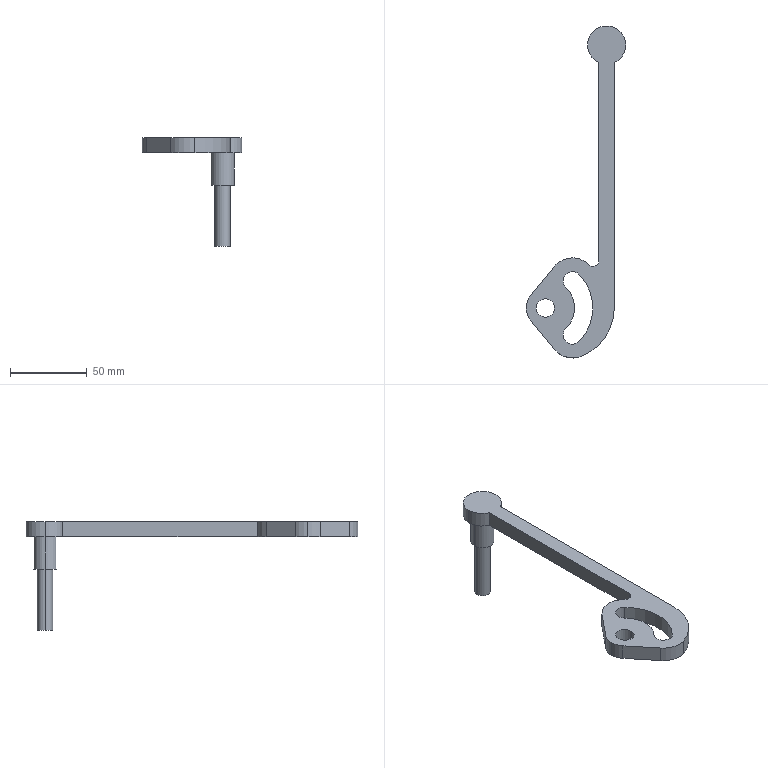Part | SolidWorks | features ICE 2, Extrusion 1 | 1 solid | 29 faces | box 65 x 216.634 x 71 mm | volume 45722 mm3 | cylinder 21 | plane 8 | commonest cylinder face diameters 12 x6 25 x5 10 x2 15 x2 30 x2 7.868 x1
STEP:
#1=CARTESIAN_POINT('',(35.,171.456,-61.));
#2=VERTEX_POINT('',#1);
#3=CARTESIAN_POINT('',(45.,171.456,-61.));
#4=VERTEX_POINT('',#3);
#5=CARTESIAN_POINT('',(40.,171.456,-61.));
#6=DIRECTION('',(0.,0.,-1.));
#7=DIRECTION('',(-1.,0.,0.));
#8=AXIS2_PLACEMENT_3D('',#5,#6,#7);
#9=CIRCLE('',#8,5.);
#10=EDGE_CURVE('',#2,#4,#9,.T.);
#11=ORIENTED_EDGE('',*,*,#10,.F.);
#12=CARTESIAN_POINT('',(35.,171.456,-21.));
#13=VERTEX_POINT('',#12);
#14=CARTESIAN_POINT('',(35.,171.456,-61.));
#15=DIRECTION('',(0.,0.,1.));
#16=VECTOR('',#15,1000.);
#17=LINE('',#14,#16);
#18=EDGE_CURVE('',#2,#13,#17,.T.);
#19=ORIENTED_EDGE('',*,*,#18,.T.);
#20=CARTESIAN_POINT('',(45.,171.456,-21.));
#21=VERTEX_POINT('',#20);
#22=CARTESIAN_POINT('',(40.,171.456,-21.));
#23=DIRECTION('',(0.,0.,-1.));
#24=DIRECTION('',(-1.,0.,0.));
#25=AXIS2_PLACEMENT_3D('',#22,#23,#24);
#26=CIRCLE('',#25,5.);
#27=EDGE_CURVE('',#13,#21,#26,.T.);
#28=ORIENTED_EDGE('',*,*,#27,.T.);
#29=CARTESIAN_POINT('',(45.,171.456,-61.));
#30=DIRECTION('',(0.,0.,1.));
#31=VECTOR('',#30,1000.);
#32=LINE('',#29,#31);
#33=EDGE_CURVE('',#4,#21,#32,.T.);
#34=ORIENTED_EDGE('',*,*,#33,.F.);
#35=EDGE_LOOP('',(#11,#19,#28,#34));
#36=FACE_OUTER_BOUND('',#35,.T.);
#37=CARTESIAN_POINT('',(40.,171.456,-61.));
#38=DIRECTION('',(0.,0.,1.));
#39=DIRECTION('',(1.,0.,0.));
#40=AXIS2_PLACEMENT_3D('',#37,#38,#39);
#41=CYLINDRICAL_SURFACE('',#40,5.);
#42=ADVANCED_FACE('',(#36),#41,.T.);
#43=CARTESIAN_POINT('',(32.5,171.456,-21.));
#44=VERTEX_POINT('',#43);
#45=CARTESIAN_POINT('',(47.5,171.456,-21.));
#46=VERTEX_POINT('',#45);
#47=CARTESIAN_POINT('',(40.,171.456,-21.));
#48=DIRECTION('',(0.,0.,-1.));
#49=DIRECTION('',(-1.,0.,0.));
#50=AXIS2_PLACEMENT_3D('',#47,#48,#49);
#51=CIRCLE('',#50,7.5);
#52=EDGE_CURVE('',#44,#46,#51,.T.);
#53=ORIENTED_EDGE('',*,*,#52,.F.);
#54=CARTESIAN_POINT('',(32.5,171.456,0.));
#55=VERTEX_POINT('',#54);
#56=CARTESIAN_POINT('',(32.5,171.456,-21.));
#57=DIRECTION('',(0.,0.,1.));
#58=VECTOR('',#57,1000.);
#59=LINE('',#56,#58);
#60=EDGE_CURVE('',#44,#55,#59,.T.);
#61=ORIENTED_EDGE('',*,*,#60,.T.);
#62=CARTESIAN_POINT('',(47.5,171.456,0.));
#63=VERTEX_POINT('',#62);
#64=CARTESIAN_POINT('',(40.,171.456,0.));
#65=DIRECTION('',(0.,0.,-1.));
#66=DIRECTION('',(1.,0.,0.));
#67=AXIS2_PLACEMENT_3D('',#64,#65,#66);
#68=CIRCLE('',#67,7.5);
#69=EDGE_CURVE('',#55,#63,#68,.T.);
#70=ORIENTED_EDGE('',*,*,#69,.T.);
#71=CARTESIAN_POINT('',(47.5,171.456,-21.));
#72=DIRECTION('',(0.,0.,1.));
#73=VECTOR('',#72,1000.);
#74=LINE('',#71,#73);
#75=EDGE_CURVE('',#46,#63,#74,.T.);
#76=ORIENTED_EDGE('',*,*,#75,.F.);
#77=EDGE_LOOP('',(#53,#61,#70,#76));
#78=FACE_OUTER_BOUND('',#77,.T.);
#79=CARTESIAN_POINT('',(40.,171.456,-21.));
#80=DIRECTION('',(0.,0.,1.));
#81=DIRECTION('',(1.,0.,0.));
#82=AXIS2_PLACEMENT_3D('',#79,#80,#81);
#83=CYLINDRICAL_SURFACE('',#82,7.5);
#84=ADVANCED_FACE('',(#78),#83,.T.);
#85=CARTESIAN_POINT('',(21.92,21.92,10.));
#86=VERTEX_POINT('',#85);
#87=CARTESIAN_POINT('',(11.678,17.678,10.));
#88=VERTEX_POINT('',#87);
#89=CARTESIAN_POINT('',(17.678,17.678,10.));
#90=DIRECTION('',(0.,0.,1.));
#91=DIRECTION('',(1.,0.,0.));
#92=AXIS2_PLACEMENT_3D('',#89,#90,#91);
#93=CIRCLE('',#92,6.);
#94=EDGE_CURVE('',#86,#88,#93,.T.);
#95=ORIENTED_EDGE('',*,*,#94,.T.);
#96=CARTESIAN_POINT('',(11.678,17.678,0.));
#97=VERTEX_POINT('',#96);
#98=CARTESIAN_POINT('',(11.678,17.678,10.));
#99=DIRECTION('',(0.,0.,-1.));
#100=VECTOR('',#99,1000.);
#101=LINE('',#98,#100);
#102=EDGE_CURVE('',#88,#97,#101,.T.);
#103=ORIENTED_EDGE('',*,*,#102,.T.);
#104=CARTESIAN_POINT('',(21.92,21.92,0.));
#105=VERTEX_POINT('',#104);
#106=CARTESIAN_POINT('',(17.678,17.678,0.));
#107=DIRECTION('',(0.,0.,1.));
#108=DIRECTION('',(1.,0.,0.));
#109=AXIS2_PLACEMENT_3D('',#106,#107,#108);
#110=CIRCLE('',#109,6.);
#111=EDGE_CURVE('',#105,#97,#110,.T.);
#112=ORIENTED_EDGE('',*,*,#111,.F.);
#113=CARTESIAN_POINT('',(21.92,21.92,10.));
#114=DIRECTION('',(0.,0.,-1.));
#115=VECTOR('',#114,1000.);
#116=LINE('',#113,#115);
#117=EDGE_CURVE('',#86,#105,#116,.T.);
#118=ORIENTED_EDGE('',*,*,#117,.F.);
#119=EDGE_LOOP('',(#95,#103,#112,#118));
#120=FACE_OUTER_BOUND('',#119,.T.);
#121=CARTESIAN_POINT('',(17.678,17.678,10.));
#122=DIRECTION('',(0.,0.,-1.));
#123=DIRECTION('',(-1.,0.,0.));
#124=AXIS2_PLACEMENT_3D('',#121,#122,#123);
#125=CYLINDRICAL_SURFACE('',#124,6.);
#126=ADVANCED_FACE('',(#120),#125,.F.);
#127=CARTESIAN_POINT('',(13.435,-13.435,10.));
#128=VERTEX_POINT('',#127);
#129=CARTESIAN_POINT('',(11.678,-17.678,10.));
#130=VERTEX_POINT('',#129);
#131=CARTESIAN_POINT('',(17.678,-17.678,10.));
#132=DIRECTION('',(0.,0.,1.));
#133=DIRECTION('',(1.,0.,0.));
#134=AXIS2_PLACEMENT_3D('',#131,#132,#133);
#135=CIRCLE('',#134,6.);
#136=EDGE_CURVE('',#128,#130,#135,.T.);
#137=ORIENTED_EDGE('',*,*,#136,.T.);
#138=CARTESIAN_POINT('',(11.678,-17.678,0.));
#139=VERTEX_POINT('',#138);
#140=CARTESIAN_POINT('',(11.678,-17.678,10.));
#141=DIRECTION('',(0.,0.,-1.));
#142=VECTOR('',#141,1000.);
#143=LINE('',#140,#142);
#144=EDGE_CURVE('',#130,#139,#143,.T.);
#145=ORIENTED_EDGE('',*,*,#144,.T.);
#146=CARTESIAN_POINT('',(13.435,-13.435,0.));
#147=VERTEX_POINT('',#146);
#148=CARTESIAN_POINT('',(17.678,-17.678,0.));
#149=DIRECTION('',(0.,0.,1.));
#150=DIRECTION('',(1.,0.,0.));
#151=AXIS2_PLACEMENT_3D('',#148,#149,#150);
#152=CIRCLE('',#151,6.);
#153=EDGE_CURVE('',#147,#139,#152,.T.);
#154=ORIENTED_EDGE('',*,*,#153,.F.);
#155=CARTESIAN_POINT('',(13.435,-13.435,10.));
#156=DIRECTION('',(0.,0.,-1.));
#157=VECTOR('',#156,1000.);
#158=LINE('',#155,#157);
#159=EDGE_CURVE('',#128,#147,#158,.T.);
#160=ORIENTED_EDGE('',*,*,#159,.F.);
#161=EDGE_LOOP('',(#137,#145,#154,#160));
#162=FACE_OUTER_BOUND('',#161,.T.);
#163=CARTESIAN_POINT('',(17.678,-17.678,10.));
#164=DIRECTION('',(0.,0.,-1.));
#165=DIRECTION('',(-1.,0.,0.));
#166=AXIS2_PLACEMENT_3D('',#163,#164,#165);
#167=CYLINDRICAL_SURFACE('',#166,6.);
#168=ADVANCED_FACE('',(#162),#167,.F.);
#169=CARTESIAN_POINT('',(-6.,0.,10.));
#170=VERTEX_POINT('',#169);
#171=CARTESIAN_POINT('',(6.,0.,10.));
#172=VERTEX_POINT('',#171);
#173=CARTESIAN_POINT('',(0.,0.,10.));
#174=DIRECTION('',(0.,0.,1.));
#175=DIRECTION('',(1.,0.,0.));
#176=AXIS2_PLACEMENT_3D('',#173,#174,#175);
#177=CIRCLE('',#176,6.);
#178=EDGE_CURVE('',#170,#172,#177,.T.);
#179=ORIENTED_EDGE('',*,*,#178,.T.);
#180=CARTESIAN_POINT('',(6.,0.,0.));
#181=VERTEX_POINT('',#180);
#182=CARTESIAN_POINT('',(6.,0.,10.));
#183=DIRECTION('',(0.,0.,-1.));
#184=VECTOR('',#183,1000.);
#185=LINE('',#182,#184);
#186=EDGE_CURVE('',#172,#181,#185,.T.);
#187=ORIENTED_EDGE('',*,*,#186,.T.);
#188=CARTESIAN_POINT('',(-6.,0.,0.));
#189=VERTEX_POINT('',#188);
#190=CARTESIAN_POINT('',(0.,0.,0.));
#191=DIRECTION('',(0.,0.,1.));
#192=DIRECTION('',(1.,0.,0.));
#193=AXIS2_PLACEMENT_3D('',#190,#191,#192);
#194=CIRCLE('',#193,6.);
#195=EDGE_CURVE('',#189,#181,#194,.T.);
#196=ORIENTED_EDGE('',*,*,#195,.F.);
#197=CARTESIAN_POINT('',(-6.,0.,10.));
#198=DIRECTION('',(0.,0.,-1.));
#199=VECTOR('',#198,1000.);
#200=LINE('',#197,#199);
#201=EDGE_CURVE('',#170,#189,#200,.T.);
#202=ORIENTED_EDGE('',*,*,#201,.F.);
#203=EDGE_LOOP('',(#179,#187,#196,#202));
#204=FACE_OUTER_BOUND('',#203,.T.);
#205=CARTESIAN_POINT('',(0.,0.,10.));
#206=DIRECTION('',(0.,0.,-1.));
#207=DIRECTION('',(-1.,0.,0.));
#208=AXIS2_PLACEMENT_3D('',#205,#206,#207);
#209=CYLINDRICAL_SURFACE('',#208,6.);
#210=ADVANCED_FACE('',(#204),#209,.F.);
#211=CARTESIAN_POINT('',(52.5,171.456,10.));
#212=VERTEX_POINT('',#211);
#213=CARTESIAN_POINT('',(27.5,171.456,10.));
#214=VERTEX_POINT('',#213);
#215=CARTESIAN_POINT('',(40.,171.456,10.));
#216=DIRECTION('',(0.,0.,1.));
#217=DIRECTION('',(1.,0.,0.));
#218=AXIS2_PLACEMENT_3D('',#215,#216,#217);
#219=CIRCLE('',#218,12.5);
#220=EDGE_CURVE('',#212,#214,#219,.T.);
#221=ORIENTED_EDGE('',*,*,#220,.F.);
#222=CARTESIAN_POINT('',(52.5,171.456,0.));
#223=VERTEX_POINT('',#222);
#224=CARTESIAN_POINT('',(52.5,171.456,10.));
#225=DIRECTION('',(0.,0.,-1.));
#226=VECTOR('',#225,1000.);
#227=LINE('',#224,#226);
#228=EDGE_CURVE('',#212,#223,#227,.T.);
#229=ORIENTED_EDGE('',*,*,#228,.T.);
#230=CARTESIAN_POINT('',(27.5,171.456,0.));
#231=VERTEX_POINT('',#230);
#232=CARTESIAN_POINT('',(40.,171.456,0.));
#233=DIRECTION('',(0.,0.,1.));
#234=DIRECTION('',(1.,0.,0.));
#235=AXIS2_PLACEMENT_3D('',#232,#233,#234);
#236=CIRCLE('',#235,12.5);
#237=EDGE_CURVE('',#223,#231,#236,.T.);
#238=ORIENTED_EDGE('',*,*,#237,.T.);
#239=CARTESIAN_POINT('',(27.5,171.456,10.));
#240=DIRECTION('',(0.,0.,-1.));
#241=VECTOR('',#240,1000.);
#242=LINE('',#239,#241);
#243=EDGE_CURVE('',#214,#231,#242,.T.);
#244=ORIENTED_EDGE('',*,*,#243,.F.);
#245=EDGE_LOOP('',(#221,#229,#238,#244));
#246=FACE_OUTER_BOUND('',#245,.T.);
#247=CARTESIAN_POINT('',(40.,171.456,10.));
#248=DIRECTION('',(0.,0.,-1.));
#249=DIRECTION('',(-1.,0.,0.));
#250=AXIS2_PLACEMENT_3D('',#247,#248,#249);
#251=CYLINDRICAL_SURFACE('',#250,12.5);
#252=ADVANCED_FACE('',(#246),#251,.T.);
#253=CARTESIAN_POINT('',(35.,160.,10.));
#254=VERTEX_POINT('',#253);
#255=CARTESIAN_POINT('',(40.,171.456,10.));
#256=DIRECTION('',(0.,0.,1.));
#257=DIRECTION('',(1.,0.,0.));
#258=AXIS2_PLACEMENT_3D('',#255,#256,#257);
#259=CIRCLE('',#258,12.5);
#260=EDGE_CURVE('',#214,#254,#259,.T.);
#261=ORIENTED_EDGE('',*,*,#260,.F.);
#262=ORIENTED_EDGE('',*,*,#243,.T.);
#263=CARTESIAN_POINT('',(35.,160.,0.));
#264=VERTEX_POINT('',#263);
#265=CARTESIAN_POINT('',(40.,171.456,0.));
#266=DIRECTION('',(0.,0.,1.));
#267=DIRECTION('',(1.,0.,0.));
#268=AXIS2_PLACEMENT_3D('',#265,#266,#267);
#269=CIRCLE('',#268,12.5);
#270=EDGE_CURVE('',#231,#264,#269,.T.);
#271=ORIENTED_EDGE('',*,*,#270,.T.);
#272=CARTESIAN_POINT('',(35.,160.,10.));
#273=DIRECTION('',(0.,0.,-1.));
#274=VECTOR('',#273,1000.);
#275=LINE('',#272,#274);
#276=EDGE_CURVE('',#254,#264,#275,.T.);
#277=ORIENTED_EDGE('',*,*,#276,.F.);
#278=EDGE_LOOP('',(#261,#262,#271,#277));
#279=FACE_OUTER_BOUND('',#278,.T.);
#280=CARTESIAN_POINT('',(40.,171.456,10.));
#281=DIRECTION('',(0.,0.,-1.));
#282=DIRECTION('',(-1.,0.,0.));
#283=AXIS2_PLACEMENT_3D('',#280,#281,#282);
#284=CYLINDRICAL_SURFACE('',#283,12.5);
#285=ADVANCED_FACE('',(#279),#284,.T.);
#286=CARTESIAN_POINT('',(-12.5,0.,10.));
#287=VERTEX_POINT('',#286);
#288=CARTESIAN_POINT('',(-9.678,-7.911,10.));
#289=VERTEX_POINT('',#288);
#290=CARTESIAN_POINT('',(0.,0.,10.));
#291=DIRECTION('',(0.,0.,1.));
#292=DIRECTION('',(1.,0.,0.));
#293=AXIS2_PLACEMENT_3D('',#290,#291,#292);
#294=CIRCLE('',#293,12.5);
#295=EDGE_CURVE('',#287,#289,#294,.T.);
#296=ORIENTED_EDGE('',*,*,#295,.F.);
#297=CARTESIAN_POINT('',(-12.5,0.,0.));
#298=VERTEX_POINT('',#297);
#299=CARTESIAN_POINT('',(-12.5,0.,10.));
#300=DIRECTION('',(0.,0.,-1.));
#301=VECTOR('',#300,1000.);
#302=LINE('',#299,#301);
#303=EDGE_CURVE('',#287,#298,#302,.T.);
#304=ORIENTED_EDGE('',*,*,#303,.T.);
#305=CARTESIAN_POINT('',(-9.678,-7.911,0.));
#306=VERTEX_POINT('',#305);
#307=CARTESIAN_POINT('',(0.,0.,0.));
#308=DIRECTION('',(0.,0.,1.));
#309=DIRECTION('',(1.,0.,0.));
#310=AXIS2_PLACEMENT_3D('',#307,#308,#309);
#311=CIRCLE('',#310,12.5);
#312=EDGE_CURVE('',#298,#306,#311,.T.);
#313=ORIENTED_EDGE('',*,*,#312,.T.);
#314=CARTESIAN_POINT('',(-9.678,-7.911,10.));
#315=DIRECTION('',(0.,0.,-1.));
#316=VECTOR('',#315,1000.);
#317=LINE('',#314,#316);
#318=EDGE_CURVE('',#289,#306,#317,.T.);
#319=ORIENTED_EDGE('',*,*,#318,.F.);
#320=EDGE_LOOP('',(#296,#304,#313,#319));
#321=FACE_OUTER_BOUND('',#320,.T.);
#322=CARTESIAN_POINT('',(0.,0.,10.));
#323=DIRECTION('',(0.,0.,-1.));
#324=DIRECTION('',(-1.,0.,0.));
#325=AXIS2_PLACEMENT_3D('',#322,#323,#324);
#326=CYLINDRICAL_SURFACE('',#325,12.5);
#327=ADVANCED_FACE('',(#321),#326,.T.);
#328=CARTESIAN_POINT('',(40.,171.456,-21.));
#329=DIRECTION('',(0.,0.,-1.));
#330=DIRECTION('',(-1.,0.,0.));
#331=AXIS2_PLACEMENT_3D('',#328,#329,#330);
#332=CIRCLE('',#331,7.5);
#333=EDGE_CURVE('',#46,#44,#332,.T.);
#334=ORIENTED_EDGE('',*,*,#333,.T.);
#335=ORIENTED_EDGE('',*,*,#52,.T.);
#336=EDGE_LOOP('',(#334,#335));
#337=FACE_OUTER_BOUND('',#336,.T.);
#338=CARTESIAN_POINT('',(40.,171.456,-21.));
#339=DIRECTION('',(0.,0.,-1.));
#340=DIRECTION('',(-1.,0.,0.));
#341=AXIS2_PLACEMENT_3D('',#338,#339,#340);
#342=CIRCLE('',#341,5.);
#343=EDGE_CURVE('',#21,#13,#342,.T.);
#344=ORIENTED_EDGE('',*,*,#343,.F.);
#345=ORIENTED_EDGE('',*,*,#27,.F.);
#346=EDGE_LOOP('',(#344,#345));
#347=FACE_BOUND('',#346,.T.);
#348=CARTESIAN_POINT('',(40.,171.456,-21.));
#349=DIRECTION('',(0.,0.,-1.));
#350=DIRECTION('',(-1.,0.,0.));
#351=AXIS2_PLACEMENT_3D('',#348,#349,#350);
#352=PLANE('',#351);
#353=ADVANCED_FACE('',(#337,#347),#352,.T.);
#354=ORIENTED_EDGE('',*,*,#153,.T.);
#355=CARTESIAN_POINT('',(21.92,-21.92,0.));
#356=VERTEX_POINT('',#355);
#357=CARTESIAN_POINT('',(17.678,-17.678,0.));
#358=DIRECTION('',(0.,0.,1.));
#359=DIRECTION('',(1.,0.,0.));
#360=AXIS2_PLACEMENT_3D('',#357,#358,#359);
#361=CIRCLE('',#360,6.);
#362=EDGE_CURVE('',#139,#356,#361,.T.);
#363=ORIENTED_EDGE('',*,*,#362,.T.);
#364=CARTESIAN_POINT('',(0.,0.,0.));
#365=DIRECTION('',(0.,0.,1.));
#366=DIRECTION('',(1.,0.,0.));
#367=AXIS2_PLACEMENT_3D('',#364,#365,#366);
#368=CIRCLE('',#367,31.);
#369=EDGE_CURVE('',#356,#105,#368,.T.);
#370=ORIENTED_EDGE('',*,*,#369,.T.);
#371=ORIENTED_EDGE('',*,*,#111,.T.);
#372=CARTESIAN_POINT('',(13.435,13.435,0.));
#373=VERTEX_POINT('',#372);
#374=CARTESIAN_POINT('',(17.678,17.678,0.));
#375=DIRECTION('',(0.,0.,1.));
#376=DIRECTION('',(1.,0.,0.));
#377=AXIS2_PLACEMENT_3D('',#374,#375,#376);
#378=CIRCLE('',#377,6.);
#379=EDGE_CURVE('',#97,#373,#378,.T.);
#380=ORIENTED_EDGE('',*,*,#379,.T.);
#381=CARTESIAN_POINT('',(0.,0.,0.));
#382=DIRECTION('',(0.,0.,-1.));
#383=DIRECTION('',(1.,0.,0.));
#384=AXIS2_PLACEMENT_3D('',#381,#382,#383);
#385=CIRCLE('',#384,19.);
#386=EDGE_CURVE('',#373,#147,#385,.T.);
#387=ORIENTED_EDGE('',*,*,#386,.T.);
#388=EDGE_LOOP('',(#354,#363,#370,#371,#380,#387));
#389=FACE_BOUND('',#388,.T.);
#390=CARTESIAN_POINT('',(35.,31.066,0.));
#391=VERTEX_POINT('',#390);
#392=CARTESIAN_POINT('',(28.284,28.284,0.));
#393=VERTEX_POINT('',#392);
#394=CARTESIAN_POINT('',(31.066,31.066,0.));
#395=DIRECTION('',(0.,0.,-1.));
#396=DIRECTION('',(1.,0.,0.));
#397=AXIS2_PLACEMENT_3D('',#394,#395,#396);
#398=CIRCLE('',#397,3.934);
#399=EDGE_CURVE('',#391,#393,#398,.T.);
#400=ORIENTED_EDGE('',*,*,#399,.F.);
#401=CARTESIAN_POINT('',(35.,160.,0.));
#402=DIRECTION('',(0.,-1.,0.));
#403=VECTOR('',#402,1000.);
#404=LINE('',#401,#403);
#405=EDGE_CURVE('',#264,#391,#404,.T.);
#406=ORIENTED_EDGE('',*,*,#405,.F.);
#407=ORIENTED_EDGE('',*,*,#270,.F.);
#408=ORIENTED_EDGE('',*,*,#237,.F.);
#409=CARTESIAN_POINT('',(45.,160.,0.));
#410=VERTEX_POINT('',#409);
#411=CARTESIAN_POINT('',(40.,171.456,0.));
#412=DIRECTION('',(0.,0.,1.));
#413=DIRECTION('',(1.,0.,0.));
#414=AXIS2_PLACEMENT_3D('',#411,#412,#413);
#415=CIRCLE('',#414,12.5);
#416=EDGE_CURVE('',#410,#223,#415,.T.);
#417=ORIENTED_EDGE('',*,*,#416,.F.);
#418=CARTESIAN_POINT('',(45.,0.,0.));
#419=VERTEX_POINT('',#418);
#420=CARTESIAN_POINT('',(45.,0.,0.));
#421=DIRECTION('',(0.,1.,0.));
#422=VECTOR('',#421,1000.);
#423=LINE('',#420,#422);
#424=EDGE_CURVE('',#419,#410,#423,.T.);
#425=ORIENTED_EDGE('',*,*,#424,.F.);
#426=CARTESIAN_POINT('',(21.92,-32.065,0.));
#427=VERTEX_POINT('',#426);
#428=CARTESIAN_POINT('',(11.186,0.,0.));
#429=DIRECTION('',(0.,0.,1.));
#430=DIRECTION('',(-1.,0.,0.));
#431=AXIS2_PLACEMENT_3D('',#428,#429,#430);
#432=CIRCLE('',#431,33.814);
#433=EDGE_CURVE('',#427,#419,#432,.T.);
#434=ORIENTED_EDGE('',*,*,#433,.F.);
#435=CARTESIAN_POINT('',(6.064,-27.17,0.));
#436=VERTEX_POINT('',#435);
#437=CARTESIAN_POINT('',(17.678,-17.678,0.));
#438=DIRECTION('',(0.,0.,1.));
#439=DIRECTION('',(1.,0.,0.));
#440=AXIS2_PLACEMENT_3D('',#437,#438,#439);
#441=CIRCLE('',#440,15.);
#442=EDGE_CURVE('',#436,#427,#441,.T.);
#443=ORIENTED_EDGE('',*,*,#442,.F.);
#444=CARTESIAN_POINT('',(-9.678,-7.911,0.));
#445=DIRECTION('',(0.6329,-0.7743,0.));
#446=VECTOR('',#445,1000.);
#447=LINE('',#444,#446);
#448=EDGE_CURVE('',#306,#436,#447,.T.);
#449=ORIENTED_EDGE('',*,*,#448,.F.);
#450=ORIENTED_EDGE('',*,*,#312,.F.);
#451=CARTESIAN_POINT('',(-9.678,7.911,0.));
#452=VERTEX_POINT('',#451);
#453=CARTESIAN_POINT('',(0.,0.,0.));
#454=DIRECTION('',(0.,0.,1.));
#455=DIRECTION('',(1.,0.,0.));
#456=AXIS2_PLACEMENT_3D('',#453,#454,#455);
#457=CIRCLE('',#456,12.5);
#458=EDGE_CURVE('',#452,#298,#457,.T.);
#459=ORIENTED_EDGE('',*,*,#458,.F.);
#460=CARTESIAN_POINT('',(6.064,27.17,0.));
#461=VERTEX_POINT('',#460);
#462=CARTESIAN_POINT('',(-9.678,7.911,0.));
#463=DIRECTION('',(-0.6329,-0.7743,0.));
#464=VECTOR('',#463,1000.);
#465=LINE('',#462,#464);
#466=EDGE_CURVE('',#461,#452,#465,.T.);
#467=ORIENTED_EDGE('',*,*,#466,.F.);
#468=CARTESIAN_POINT('',(17.678,17.678,0.));
#469=DIRECTION('',(0.,0.,1.));
#470=DIRECTION('',(1.,0.,0.));
#471=AXIS2_PLACEMENT_3D('',#468,#469,#470);
#472=CIRCLE('',#471,15.);
#473=EDGE_CURVE('',#393,#461,#472,.T.);
#474=ORIENTED_EDGE('',*,*,#473,.F.);
#475=EDGE_LOOP('',(#400,#406,#407,#408,#417,#425,#434,#443,#449,#450,#459,#467,#474));
#476=FACE_OUTER_BOUND('',#475,.T.);
#477=ORIENTED_EDGE('',*,*,#195,.T.);
#478=CARTESIAN_POINT('',(0.,0.,0.));
#479=DIRECTION('',(0.,0.,1.));
#480=DIRECTION('',(1.,0.,0.));
#481=AXIS2_PLACEMENT_3D('',#478,#479,#480);
#482=CIRCLE('',#481,6.);
#483=EDGE_CURVE('',#181,#189,#482,.T.);
#484=ORIENTED_EDGE('',*,*,#483,.T.);
#485=EDGE_LOOP('',(#477,#484));
#486=FACE_BOUND('',#485,.T.);
#487=CARTESIAN_POINT('',(40.,171.456,0.));
#488=DIRECTION('',(0.,0.,-1.));
#489=DIRECTION('',(1.,0.,0.));
#490=AXIS2_PLACEMENT_3D('',#487,#488,#489);
#491=CIRCLE('',#490,7.5);
#492=EDGE_CURVE('',#63,#55,#491,.T.);
#493=ORIENTED_EDGE('',*,*,#492,.F.);
#494=ORIENTED_EDGE('',*,*,#69,.F.);
#495=EDGE_LOOP('',(#493,#494));
#496=FACE_BOUND('',#495,.T.);
#497=CARTESIAN_POINT('',(31.066,31.066,0.));
#498=DIRECTION('',(0.,0.,1.));
#499=DIRECTION('',(1.,0.,0.));
#500=AXIS2_PLACEMENT_3D('',#497,#498,#499);
#501=PLANE('',#500);
#502=ADVANCED_FACE('',(#389,#476,#486,#496),#501,.F.);
#503=ORIENTED_EDGE('',*,*,#178,.F.);
#504=CARTESIAN_POINT('',(0.,0.,10.));
#505=DIRECTION('',(0.,0.,1.));
#506=DIRECTION('',(1.,0.,0.));
#507=AXIS2_PLACEMENT_3D('',#504,#505,#506);
#508=CIRCLE('',#507,6.);
#509=EDGE_CURVE('',#172,#170,#508,.T.);
#510=ORIENTED_EDGE('',*,*,#509,.F.);
#511=EDGE_LOOP('',(#503,#510));
#512=FACE_BOUND('',#511,.T.);
#513=CARTESIAN_POINT('',(35.,31.066,10.));
#514=VERTEX_POINT('',#513);
#515=CARTESIAN_POINT('',(28.284,28.284,10.));
#516=VERTEX_POINT('',#515);
#517=CARTESIAN_POINT('',(31.066,31.066,10.));
#518=DIRECTION('',(0.,0.,-1.));
#519=DIRECTION('',(1.,0.,0.));
#520=AXIS2_PLACEMENT_3D('',#517,#518,#519);
#521=CIRCLE('',#520,3.934);
#522=EDGE_CURVE('',#514,#516,#521,.T.);
#523=ORIENTED_EDGE('',*,*,#522,.T.);
#524=CARTESIAN_POINT('',(6.064,27.17,10.));
#525=VERTEX_POINT('',#524);
#526=CARTESIAN_POINT('',(17.678,17.678,10.));
#527=DIRECTION('',(0.,0.,1.));
#528=DIRECTION('',(1.,0.,0.));
#529=AXIS2_PLACEMENT_3D('',#526,#527,#528);
#530=CIRCLE('',#529,15.);
#531=EDGE_CURVE('',#516,#525,#530,.T.);
#532=ORIENTED_EDGE('',*,*,#531,.T.);
#533=CARTESIAN_POINT('',(-9.678,7.911,10.));
#534=VERTEX_POINT('',#533);
#535=CARTESIAN_POINT('',(-9.678,7.911,10.));
#536=DIRECTION('',(-0.6329,-0.7743,0.));
#537=VECTOR('',#536,1000.);
#538=LINE('',#535,#537);
#539=EDGE_CURVE('',#525,#534,#538,.T.);
#540=ORIENTED_EDGE('',*,*,#539,.T.);
#541=CARTESIAN_POINT('',(0.,0.,10.));
#542=DIRECTION('',(0.,0.,1.));
#543=DIRECTION('',(1.,0.,0.));
#544=AXIS2_PLACEMENT_3D('',#541,#542,#543);
#545=CIRCLE('',#544,12.5);
#546=EDGE_CURVE('',#534,#287,#545,.T.);
#547=ORIENTED_EDGE('',*,*,#546,.T.);
#548=ORIENTED_EDGE('',*,*,#295,.T.);
#549=CARTESIAN_POINT('',(6.064,-27.17,10.));
#550=VERTEX_POINT('',#549);
#551=CARTESIAN_POINT('',(-9.678,-7.911,10.));
#552=DIRECTION('',(0.6329,-0.7743,0.));
#553=VECTOR('',#552,1000.);
#554=LINE('',#551,#553);
#555=EDGE_CURVE('',#289,#550,#554,.T.);
#556=ORIENTED_EDGE('',*,*,#555,.T.);
#557=CARTESIAN_POINT('',(21.92,-32.065,10.));
#558=VERTEX_POINT('',#557);
#559=CARTESIAN_POINT('',(17.678,-17.678,10.));
#560=DIRECTION('',(0.,0.,1.));
#561=DIRECTION('',(1.,0.,0.));
#562=AXIS2_PLACEMENT_3D('',#559,#560,#561);
#563=CIRCLE('',#562,15.);
#564=EDGE_CURVE('',#550,#558,#563,.T.);
#565=ORIENTED_EDGE('',*,*,#564,.T.);
#566=CARTESIAN_POINT('',(45.,0.,10.));
#567=VERTEX_POINT('',#566);
#568=CARTESIAN_POINT('',(11.186,0.,10.));
#569=DIRECTION('',(0.,0.,1.));
#570=DIRECTION('',(-1.,0.,0.));
#571=AXIS2_PLACEMENT_3D('',#568,#569,#570);
#572=CIRCLE('',#571,33.814);
#573=EDGE_CURVE('',#558,#567,#572,.T.);
#574=ORIENTED_EDGE('',*,*,#573,.T.);
#575=CARTESIAN_POINT('',(45.,160.,10.));
#576=VERTEX_POINT('',#575);
#577=CARTESIAN_POINT('',(45.,0.,10.));
#578=DIRECTION('',(0.,1.,0.));
#579=VECTOR('',#578,1000.);
#580=LINE('',#577,#579);
#581=EDGE_CURVE('',#567,#576,#580,.T.);
#582=ORIENTED_EDGE('',*,*,#581,.T.);
#583=CARTESIAN_POINT('',(40.,171.456,10.));
#584=DIRECTION('',(0.,0.,1.));
#585=DIRECTION('',(1.,0.,0.));
#586=AXIS2_PLACEMENT_3D('',#583,#584,#585);
#587=CIRCLE('',#586,12.5);
#588=EDGE_CURVE('',#576,#212,#587,.T.);
#589=ORIENTED_EDGE('',*,*,#588,.T.);
#590=ORIENTED_EDGE('',*,*,#220,.T.);
#591=ORIENTED_EDGE('',*,*,#260,.T.);
#592=CARTESIAN_POINT('',(35.,160.,10.));
#593=DIRECTION('',(0.,-1.,0.));
#594=VECTOR('',#593,1000.);
#595=LINE('',#592,#594);
#596=EDGE_CURVE('',#254,#514,#595,.T.);
#597=ORIENTED_EDGE('',*,*,#596,.T.);
#598=EDGE_LOOP('',(#523,#532,#540,#547,#548,#556,#565,#574,#582,#589,#590,#591,#597));
#599=FACE_OUTER_BOUND('',#598,.T.);
#600=CARTESIAN_POINT('',(21.92,-21.92,10.));
#601=VERTEX_POINT('',#600);
#602=CARTESIAN_POINT('',(0.,0.,10.));
#603=DIRECTION('',(0.,0.,1.));
#604=DIRECTION('',(1.,0.,0.));
#605=AXIS2_PLACEMENT_3D('',#602,#603,#604);
#606=CIRCLE('',#605,31.);
#607=EDGE_CURVE('',#601,#86,#606,.T.);
#608=ORIENTED_EDGE('',*,*,#607,.F.);
#609=CARTESIAN_POINT('',(17.678,-17.678,10.));
#610=DIRECTION('',(0.,0.,1.));
#611=DIRECTION('',(1.,0.,0.));
#612=AXIS2_PLACEMENT_3D('',#609,#610,#611);
#613=CIRCLE('',#612,6.);
#614=EDGE_CURVE('',#130,#601,#613,.T.);
#615=ORIENTED_EDGE('',*,*,#614,.F.);
#616=ORIENTED_EDGE('',*,*,#136,.F.);
#617=CARTESIAN_POINT('',(13.435,13.435,10.));
#618=VERTEX_POINT('',#617);
#619=CARTESIAN_POINT('',(0.,0.,10.));
#620=DIRECTION('',(0.,0.,-1.));
#621=DIRECTION('',(1.,0.,0.));
#622=AXIS2_PLACEMENT_3D('',#619,#620,#621);
#623=CIRCLE('',#622,19.);
#624=EDGE_CURVE('',#618,#128,#623,.T.);
#625=ORIENTED_EDGE('',*,*,#624,.F.);
#626=CARTESIAN_POINT('',(17.678,17.678,10.));
#627=DIRECTION('',(0.,0.,1.));
#628=DIRECTION('',(1.,0.,0.));
#629=AXIS2_PLACEMENT_3D('',#626,#627,#628);
#630=CIRCLE('',#629,6.);
#631=EDGE_CURVE('',#88,#618,#630,.T.);
#632=ORIENTED_EDGE('',*,*,#631,.F.);
#633=ORIENTED_EDGE('',*,*,#94,.F.);
#634=EDGE_LOOP('',(#608,#615,#616,#625,#632,#633));
#635=FACE_BOUND('',#634,.T.);
#636=CARTESIAN_POINT('',(31.066,31.066,10.));
#637=DIRECTION('',(0.,0.,1.));
#638=DIRECTION('',(1.,0.,0.));
#639=AXIS2_PLACEMENT_3D('',#636,#637,#638);
#640=PLANE('',#639);
#641=ADVANCED_FACE('',(#512,#599,#635),#640,.T.);
#642=ORIENTED_EDGE('',*,*,#399,.T.);
#643=CARTESIAN_POINT('',(28.284,28.284,10.));
#644=DIRECTION('',(0.,0.,-1.));
#645=VECTOR('',#644,1000.);
#646=LINE('',#643,#645);
#647=EDGE_CURVE('',#516,#393,#646,.T.);
#648=ORIENTED_EDGE('',*,*,#647,.F.);
#649=ORIENTED_EDGE('',*,*,#522,.F.);
#650=CARTESIAN_POINT('',(35.,31.066,10.));
#651=DIRECTION('',(0.,0.,-1.));
#652=VECTOR('',#651,1000.);
#653=LINE('',#650,#652);
#654=EDGE_CURVE('',#514,#391,#653,.T.);
#655=ORIENTED_EDGE('',*,*,#654,.T.);
#656=EDGE_LOOP('',(#642,#648,#649,#655));
#657=FACE_OUTER_BOUND('',#656,.T.);
#658=CARTESIAN_POINT('',(31.066,31.066,10.));
#659=DIRECTION('',(0.,0.,-1.));
#660=DIRECTION('',(-1.,0.,0.));
#661=AXIS2_PLACEMENT_3D('',#658,#659,#660);
#662=CYLINDRICAL_SURFACE('',#661,3.934);
#663=ADVANCED_FACE('',(#657),#662,.F.);
#664=ORIENTED_EDGE('',*,*,#473,.T.);
#665=CARTESIAN_POINT('',(6.064,27.17,10.));
#666=DIRECTION('',(0.,0.,-1.));
#667=VECTOR('',#666,1000.);
#668=LINE('',#665,#667);
#669=EDGE_CURVE('',#525,#461,#668,.T.);
#670=ORIENTED_EDGE('',*,*,#669,.F.);
#671=ORIENTED_EDGE('',*,*,#531,.F.);
#672=ORIENTED_EDGE('',*,*,#647,.T.);
#673=EDGE_LOOP('',(#664,#670,#671,#672));
#674=FACE_OUTER_BOUND('',#673,.T.);
#675=CARTESIAN_POINT('',(17.678,17.678,10.));
#676=DIRECTION('',(0.,0.,-1.));
#677=DIRECTION('',(-1.,0.,0.));
#678=AXIS2_PLACEMENT_3D('',#675,#676,#677);
#679=CYLINDRICAL_SURFACE('',#678,15.);
#680=ADVANCED_FACE('',(#674),#679,.T.);
#681=ORIENTED_EDGE('',*,*,#466,.T.);
#682=CARTESIAN_POINT('',(-9.678,7.911,10.));
#683=DIRECTION('',(0.,0.,-1.));
#684=VECTOR('',#683,1000.);
#685=LINE('',#682,#684);
#686=EDGE_CURVE('',#534,#452,#685,.T.);
#687=ORIENTED_EDGE('',*,*,#686,.F.);
#688=ORIENTED_EDGE('',*,*,#539,.F.);
#689=ORIENTED_EDGE('',*,*,#669,.T.);
#690=EDGE_LOOP('',(#681,#687,#688,#689));
#691=FACE_OUTER_BOUND('',#690,.T.);
#692=CARTESIAN_POINT('',(-9.678,7.911,10.));
#693=DIRECTION('',(0.7743,-0.6329,0.));
#694=DIRECTION('',(0.6329,0.7743,0.));
#695=AXIS2_PLACEMENT_3D('',#692,#693,#694);
#696=PLANE('',#695);
#697=ADVANCED_FACE('',(#691),#696,.F.);
#698=ORIENTED_EDGE('',*,*,#303,.F.);
#699=ORIENTED_EDGE('',*,*,#546,.F.);
#700=ORIENTED_EDGE('',*,*,#686,.T.);
#701=ORIENTED_EDGE('',*,*,#458,.T.);
#702=EDGE_LOOP('',(#698,#699,#700,#701));
#703=FACE_OUTER_BOUND('',#702,.T.);
#704=CARTESIAN_POINT('',(0.,0.,10.));
#705=DIRECTION('',(0.,0.,-1.));
#706=DIRECTION('',(-1.,0.,0.));
#707=AXIS2_PLACEMENT_3D('',#704,#705,#706);
#708=CYLINDRICAL_SURFACE('',#707,12.5);
#709=ADVANCED_FACE('',(#703),#708,.T.);
#710=ORIENTED_EDGE('',*,*,#448,.T.);
#711=CARTESIAN_POINT('',(6.064,-27.17,10.));
#712=DIRECTION('',(0.,0.,-1.));
#713=VECTOR('',#712,1000.);
#714=LINE('',#711,#713);
#715=EDGE_CURVE('',#550,#436,#714,.T.);
#716=ORIENTED_EDGE('',*,*,#715,.F.);
#717=ORIENTED_EDGE('',*,*,#555,.F.);
#718=ORIENTED_EDGE('',*,*,#318,.T.);
#719=EDGE_LOOP('',(#710,#716,#717,#718));
#720=FACE_OUTER_BOUND('',#719,.T.);
#721=CARTESIAN_POINT('',(-9.678,-7.911,10.));
#722=DIRECTION('',(0.7743,0.6329,0.));
#723=DIRECTION('',(-0.6329,0.7743,0.));
#724=AXIS2_PLACEMENT_3D('',#721,#722,#723);
#725=PLANE('',#724);
#726=ADVANCED_FACE('',(#720),#725,.F.);
#727=ORIENTED_EDGE('',*,*,#442,.T.);
#728=CARTESIAN_POINT('',(21.92,-32.065,10.));
#729=DIRECTION('',(0.,0.,-1.));
#730=VECTOR('',#729,1000.);
#731=LINE('',#728,#730);
#732=EDGE_CURVE('',#558,#427,#731,.T.);
#733=ORIENTED_EDGE('',*,*,#732,.F.);
#734=ORIENTED_EDGE('',*,*,#564,.F.);
#735=ORIENTED_EDGE('',*,*,#715,.T.);
#736=EDGE_LOOP('',(#727,#733,#734,#735));
#737=FACE_OUTER_BOUND('',#736,.T.);
#738=CARTESIAN_POINT('',(17.678,-17.678,10.));
#739=DIRECTION('',(0.,0.,-1.));
#740=DIRECTION('',(-1.,0.,0.));
#741=AXIS2_PLACEMENT_3D('',#738,#739,#740);
#742=CYLINDRICAL_SURFACE('',#741,15.);
#743=ADVANCED_FACE('',(#737),#742,.T.);
#744=ORIENTED_EDGE('',*,*,#433,.T.);
#745=CARTESIAN_POINT('',(45.,0.,10.));
#746=DIRECTION('',(0.,0.,-1.));
#747=VECTOR('',#746,1000.);
#748=LINE('',#745,#747);
#749=EDGE_CURVE('',#567,#419,#748,.T.);
#750=ORIENTED_EDGE('',*,*,#749,.F.);
#751=ORIENTED_EDGE('',*,*,#573,.F.);
#752=ORIENTED_EDGE('',*,*,#732,.T.);
#753=EDGE_LOOP('',(#744,#750,#751,#752));
#754=FACE_OUTER_BOUND('',#753,.T.);
#755=CARTESIAN_POINT('',(11.186,0.,10.));
#756=DIRECTION('',(0.,0.,-1.));
#757=DIRECTION('',(-1.,0.,0.));
#758=AXIS2_PLACEMENT_3D('',#755,#756,#757);
#759=CYLINDRICAL_SURFACE('',#758,33.814);
#760=ADVANCED_FACE('',(#754),#759,.T.);
#761=ORIENTED_EDGE('',*,*,#424,.T.);
#762=CARTESIAN_POINT('',(45.,160.,10.));
#763=DIRECTION('',(0.,0.,-1.));
#764=VECTOR('',#763,1000.);
#765=LINE('',#762,#764);
#766=EDGE_CURVE('',#576,#410,#765,.T.);
#767=ORIENTED_EDGE('',*,*,#766,.F.);
#768=ORIENTED_EDGE('',*,*,#581,.F.);
#769=ORIENTED_EDGE('',*,*,#749,.T.);
#770=EDGE_LOOP('',(#761,#767,#768,#769));
#771=FACE_OUTER_BOUND('',#770,.T.);
#772=CARTESIAN_POINT('',(45.,0.,10.));
#773=DIRECTION('',(-1.,0.,0.));
#774=DIRECTION('',(0.,0.,1.));
#775=AXIS2_PLACEMENT_3D('',#772,#773,#774);
#776=PLANE('',#775);
#777=ADVANCED_FACE('',(#771),#776,.F.);
#778=ORIENTED_EDGE('',*,*,#228,.F.);
#779=ORIENTED_EDGE('',*,*,#588,.F.);
#780=ORIENTED_EDGE('',*,*,#766,.T.);
#781=ORIENTED_EDGE('',*,*,#416,.T.);
#782=EDGE_LOOP('',(#778,#779,#780,#781));
#783=FACE_OUTER_BOUND('',#782,.T.);
#784=CARTESIAN_POINT('',(40.,171.456,10.));
#785=DIRECTION('',(0.,0.,-1.));
#786=DIRECTION('',(-1.,0.,0.));
#787=AXIS2_PLACEMENT_3D('',#784,#785,#786);
#788=CYLINDRICAL_SURFACE('',#787,12.5);
#789=ADVANCED_FACE('',(#783),#788,.T.);
#790=ORIENTED_EDGE('',*,*,#405,.T.);
#791=ORIENTED_EDGE('',*,*,#654,.F.);
#792=ORIENTED_EDGE('',*,*,#596,.F.);
#793=ORIENTED_EDGE('',*,*,#276,.T.);
#794=EDGE_LOOP('',(#790,#791,#792,#793));
#795=FACE_OUTER_BOUND('',#794,.T.);
#796=CARTESIAN_POINT('',(35.,160.,10.));
#797=DIRECTION('',(1.,0.,0.));
#798=DIRECTION('',(0.,1.,0.));
#799=AXIS2_PLACEMENT_3D('',#796,#797,#798);
#800=PLANE('',#799);
#801=ADVANCED_FACE('',(#795),#800,.F.);
#802=ORIENTED_EDGE('',*,*,#186,.F.);
#803=ORIENTED_EDGE('',*,*,#509,.T.);
#804=ORIENTED_EDGE('',*,*,#201,.T.);
#805=ORIENTED_EDGE('',*,*,#483,.F.);
#806=EDGE_LOOP('',(#802,#803,#804,#805));
#807=FACE_OUTER_BOUND('',#806,.T.);
#808=CARTESIAN_POINT('',(0.,0.,10.));
#809=DIRECTION('',(0.,0.,-1.));
#810=DIRECTION('',(-1.,0.,0.));
#811=AXIS2_PLACEMENT_3D('',#808,#809,#810);
#812=CYLINDRICAL_SURFACE('',#811,6.);
#813=ADVANCED_FACE('',(#807),#812,.F.);
#814=ORIENTED_EDGE('',*,*,#144,.F.);
#815=ORIENTED_EDGE('',*,*,#614,.T.);
#816=CARTESIAN_POINT('',(21.92,-21.92,10.));
#817=DIRECTION('',(0.,0.,-1.));
#818=VECTOR('',#817,1000.);
#819=LINE('',#816,#818);
#820=EDGE_CURVE('',#601,#356,#819,.T.);
#821=ORIENTED_EDGE('',*,*,#820,.T.);
#822=ORIENTED_EDGE('',*,*,#362,.F.);
#823=EDGE_LOOP('',(#814,#815,#821,#822));
#824=FACE_OUTER_BOUND('',#823,.T.);
#825=CARTESIAN_POINT('',(17.678,-17.678,10.));
#826=DIRECTION('',(0.,0.,-1.));
#827=DIRECTION('',(-1.,0.,0.));
#828=AXIS2_PLACEMENT_3D('',#825,#826,#827);
#829=CYLINDRICAL_SURFACE('',#828,6.);
#830=ADVANCED_FACE('',(#824),#829,.F.);
#831=ORIENTED_EDGE('',*,*,#369,.F.);
#832=ORIENTED_EDGE('',*,*,#820,.F.);
#833=ORIENTED_EDGE('',*,*,#607,.T.);
#834=ORIENTED_EDGE('',*,*,#117,.T.);
#835=EDGE_LOOP('',(#831,#832,#833,#834));
#836=FACE_OUTER_BOUND('',#835,.T.);
#837=CARTESIAN_POINT('',(0.,0.,10.));
#838=DIRECTION('',(0.,0.,-1.));
#839=DIRECTION('',(-1.,0.,0.));
#840=AXIS2_PLACEMENT_3D('',#837,#838,#839);
#841=CYLINDRICAL_SURFACE('',#840,31.);
#842=ADVANCED_FACE('',(#836),#841,.F.);
#843=ORIENTED_EDGE('',*,*,#102,.F.);
#844=ORIENTED_EDGE('',*,*,#631,.T.);
#845=CARTESIAN_POINT('',(13.435,13.435,10.));
#846=DIRECTION('',(0.,0.,-1.));
#847=VECTOR('',#846,1000.);
#848=LINE('',#845,#847);
#849=EDGE_CURVE('',#618,#373,#848,.T.);
#850=ORIENTED_EDGE('',*,*,#849,.T.);
#851=ORIENTED_EDGE('',*,*,#379,.F.);
#852=EDGE_LOOP('',(#843,#844,#850,#851));
#853=FACE_OUTER_BOUND('',#852,.T.);
#854=CARTESIAN_POINT('',(17.678,17.678,10.));
#855=DIRECTION('',(0.,0.,-1.));
#856=DIRECTION('',(-1.,0.,0.));
#857=AXIS2_PLACEMENT_3D('',#854,#855,#856);
#858=CYLINDRICAL_SURFACE('',#857,6.);
#859=ADVANCED_FACE('',(#853),#858,.F.);
#860=ORIENTED_EDGE('',*,*,#386,.F.);
#861=ORIENTED_EDGE('',*,*,#849,.F.);
#862=ORIENTED_EDGE('',*,*,#624,.T.);
#863=ORIENTED_EDGE('',*,*,#159,.T.);
#864=EDGE_LOOP('',(#860,#861,#862,#863));
#865=FACE_OUTER_BOUND('',#864,.T.);
#866=CARTESIAN_POINT('',(0.,0.,10.));
#867=DIRECTION('',(0.,0.,-1.));
#868=DIRECTION('',(-1.,0.,0.));
#869=AXIS2_PLACEMENT_3D('',#866,#867,#868);
#870=CYLINDRICAL_SURFACE('',#869,19.);
#871=ADVANCED_FACE('',(#865),#870,.T.);
#872=ORIENTED_EDGE('',*,*,#60,.F.);
#873=ORIENTED_EDGE('',*,*,#333,.F.);
#874=ORIENTED_EDGE('',*,*,#75,.T.);
#875=ORIENTED_EDGE('',*,*,#492,.T.);
#876=EDGE_LOOP('',(#872,#873,#874,#875));
#877=FACE_OUTER_BOUND('',#876,.T.);
#878=CARTESIAN_POINT('',(40.,171.456,-21.));
#879=DIRECTION('',(0.,0.,1.));
#880=DIRECTION('',(1.,0.,0.));
#881=AXIS2_PLACEMENT_3D('',#878,#879,#880);
#882=CYLINDRICAL_SURFACE('',#881,7.5);
#883=ADVANCED_FACE('',(#877),#882,.T.);
#884=ORIENTED_EDGE('',*,*,#18,.F.);
#885=CARTESIAN_POINT('',(40.,171.456,-61.));
#886=DIRECTION('',(0.,0.,-1.));
#887=DIRECTION('',(-1.,0.,0.));
#888=AXIS2_PLACEMENT_3D('',#885,#886,#887);
#889=CIRCLE('',#888,5.);
#890=EDGE_CURVE('',#4,#2,#889,.T.);
#891=ORIENTED_EDGE('',*,*,#890,.F.);
#892=ORIENTED_EDGE('',*,*,#33,.T.);
#893=ORIENTED_EDGE('',*,*,#343,.T.);
#894=EDGE_LOOP('',(#884,#891,#892,#893));
#895=FACE_OUTER_BOUND('',#894,.T.);
#896=CARTESIAN_POINT('',(40.,171.456,-61.));
#897=DIRECTION('',(0.,0.,1.));
#898=DIRECTION('',(1.,0.,0.));
#899=AXIS2_PLACEMENT_3D('',#896,#897,#898);
#900=CYLINDRICAL_SURFACE('',#899,5.);
#901=ADVANCED_FACE('',(#895),#900,.T.);
#902=ORIENTED_EDGE('',*,*,#890,.T.);
#903=ORIENTED_EDGE('',*,*,#10,.T.);
#904=EDGE_LOOP('',(#902,#903));
#905=FACE_OUTER_BOUND('',#904,.T.);
#906=CARTESIAN_POINT('',(40.,171.456,-61.));
#907=DIRECTION('',(0.,0.,-1.));
#908=DIRECTION('',(-1.,0.,0.));
#909=AXIS2_PLACEMENT_3D('',#906,#907,#908);
#910=PLANE('',#909);
#911=ADVANCED_FACE('',(#905),#910,.T.);
#912=CLOSED_SHELL('',(#42,#84,#126,#168,#210,#252,#285,#327,#353,#502,#641,#663,#680,#697,#709,#726,#743,#760,#777,#789,#801,#813,#830,#842,#859,#871,#883,#901,#911));
#913=MANIFOLD_SOLID_BREP('',#912);
#914=CARTESIAN_POINT('',(0.,0.,0.));
#915=DIRECTION('',(0.,0.,1.));
#916=DIRECTION('',(1.,0.,0.));
#917=AXIS2_PLACEMENT_3D('',#914,#915,#916);
#918=(LENGTH_UNIT()NAMED_UNIT(*)SI_UNIT(.MILLI.,.METRE.));
#919=UNCERTAINTY_MEASURE_WITH_UNIT(LENGTH_MEASURE(0.00001),#918,'','');
#920=(NAMED_UNIT(*)PLANE_ANGLE_UNIT()SI_UNIT($,.RADIAN.));
#921=(NAMED_UNIT(*)SI_UNIT($,.STERADIAN.)SOLID_ANGLE_UNIT());
#922=(GEOMETRIC_REPRESENTATION_CONTEXT(3)GLOBAL_UNCERTAINTY_ASSIGNED_CONTEXT((#919))GLOBAL_UNIT_ASSIGNED_CONTEXT((#918,#920,#921))REPRESENTATION_CONTEXT('',''));
#923=ADVANCED_BREP_SHAPE_REPRESENTATION('',(#913,#917),#922);